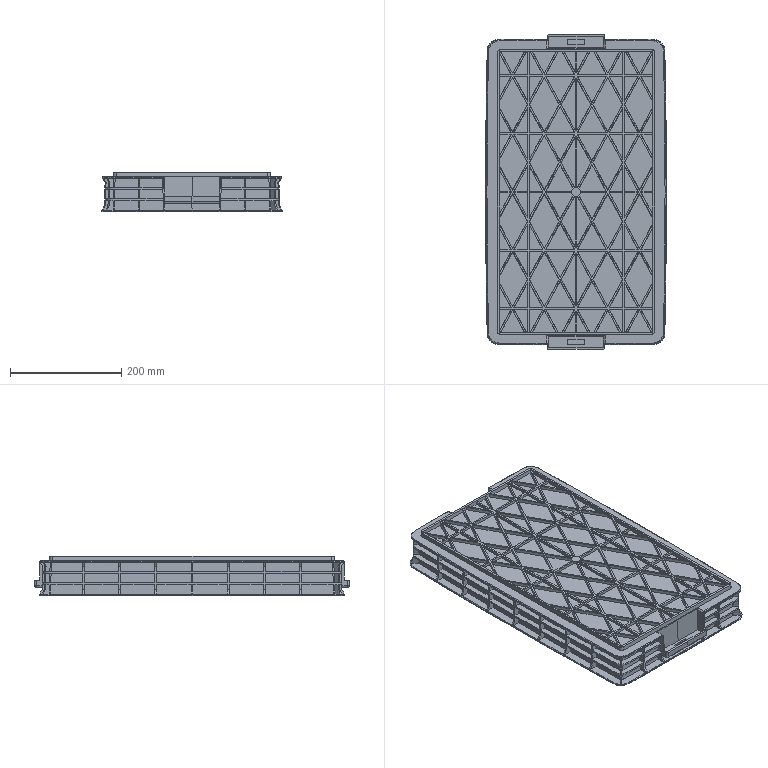Part | SolidWorks | features BaseBody 1 | 1 solid | 1340 faces | box 324.683 x 565.23 x 71 mm | volume 1485428 mm3 | plane 959 | spline 206 | cone 89 | torus 49 | cylinder 33 | sphere 4 | commonest cylinder face diameters 6 x8 16 x8 22228 x5 4 x4 10 x4 40 x4